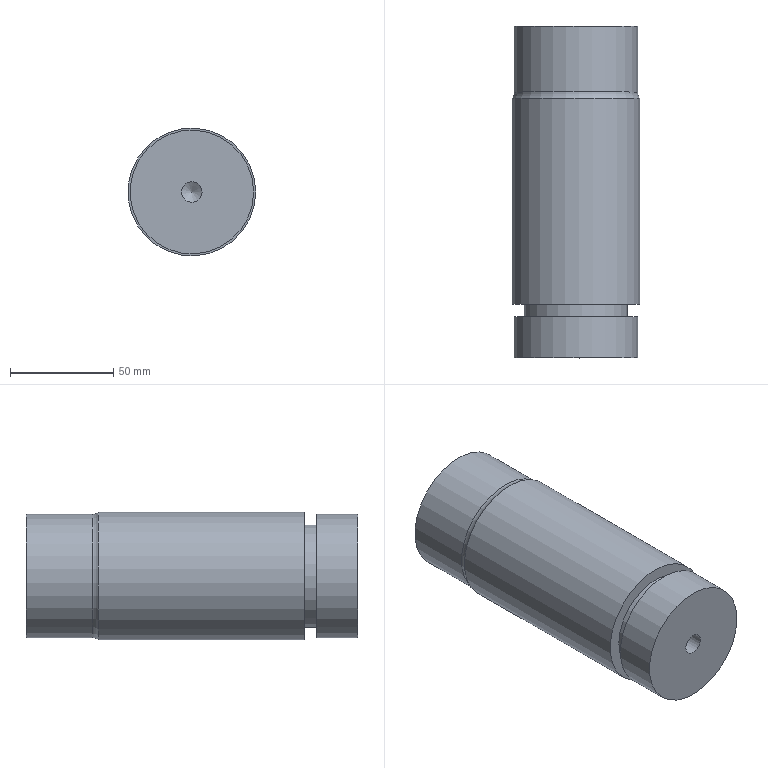Part | NX | features MAIN_BODY 2 | 1 solid | 11 faces | box 62 x 161 x 62 mm | volume 467651 mm3 | cylinder 5 | plane 4 | torus 1 | cone 1 | commonest cylinder face diameters 60 x2 10 x1 50 x1 62 x1
STEP:
#1=CARTESIAN_POINT('',(445.,-617.,262.));
#2=VERTEX_POINT('',#1);
#3=CARTESIAN_POINT('',(414.,-617.,262.));
#4=DIRECTION('',(0.,-1.,0.));
#5=DIRECTION('',(1.,0.,0.));
#6=AXIS2_PLACEMENT_3D('',#3,#4,#5);
#7=CIRCLE('',#6,31.);
#8=EDGE_CURVE('',#2,#2,#7,.T.);
#9=ORIENTED_EDGE('',*,*,#8,.F.);
#10=EDGE_LOOP('',(#9));
#11=FACE_BOUND('',#10,.T.);
#12=CARTESIAN_POINT('',(445.,-517.,262.));
#13=VERTEX_POINT('',#12);
#14=CARTESIAN_POINT('',(414.,-517.,262.));
#15=DIRECTION('',(0.,-1.,0.));
#16=DIRECTION('',(1.,0.,0.));
#17=AXIS2_PLACEMENT_3D('',#14,#15,#16);
#18=CIRCLE('',#17,31.);
#19=EDGE_CURVE('',#13,#13,#18,.T.);
#20=ORIENTED_EDGE('',*,*,#19,.T.);
#21=EDGE_LOOP('',(#20));
#22=FACE_BOUND('',#21,.T.);
#23=CARTESIAN_POINT('',(414.,-617.,262.));
#24=DIRECTION('',(0.,1.,0.));
#25=DIRECTION('',(-1.,0.,0.));
#26=AXIS2_PLACEMENT_3D('',#23,#24,#25);
#27=CYLINDRICAL_SURFACE('',#26,31.);
#28=ADVANCED_FACE('',(#11,#22),#27,.T.);
#29=CARTESIAN_POINT('',(439.,-617.,262.));
#30=VERTEX_POINT('',#29);
#31=CARTESIAN_POINT('',(414.,-617.,262.));
#32=DIRECTION('',(0.,-1.,0.));
#33=DIRECTION('',(1.,0.,0.));
#34=AXIS2_PLACEMENT_3D('',#31,#32,#33);
#35=CIRCLE('',#34,25.);
#36=EDGE_CURVE('',#30,#30,#35,.T.);
#37=ORIENTED_EDGE('',*,*,#36,.F.);
#38=EDGE_LOOP('',(#37));
#39=FACE_BOUND('',#38,.T.);
#40=ORIENTED_EDGE('',*,*,#8,.T.);
#41=EDGE_LOOP('',(#40));
#42=FACE_BOUND('',#41,.T.);
#43=CARTESIAN_POINT('',(414.,-617.,262.));
#44=DIRECTION('',(0.,-1.,0.));
#45=DIRECTION('',(1.,0.,0.));
#46=AXIS2_PLACEMENT_3D('',#43,#44,#45);
#47=PLANE('',#46);
#48=ADVANCED_FACE('',(#39,#42),#47,.T.);
#49=CARTESIAN_POINT('',(444.,-514.,262.));
#50=VERTEX_POINT('',#49);
#51=CARTESIAN_POINT('',(414.,-514.,262.));
#52=DIRECTION('',(0.,-1.,0.));
#53=DIRECTION('',(1.,0.,0.));
#54=AXIS2_PLACEMENT_3D('',#51,#52,#53);
#55=CIRCLE('',#54,30.);
#56=EDGE_CURVE('',#50,#50,#55,.F.);
#57=ORIENTED_EDGE('',*,*,#56,.T.);
#58=EDGE_LOOP('',(#57));
#59=FACE_BOUND('',#58,.T.);
#60=CARTESIAN_POINT('',(444.,-482.,262.));
#61=VERTEX_POINT('',#60);
#62=CARTESIAN_POINT('',(414.,-482.,262.));
#63=DIRECTION('',(0.,-1.,0.));
#64=DIRECTION('',(1.,0.,0.));
#65=AXIS2_PLACEMENT_3D('',#62,#63,#64);
#66=CIRCLE('',#65,30.);
#67=EDGE_CURVE('',#61,#61,#66,.T.);
#68=ORIENTED_EDGE('',*,*,#67,.T.);
#69=EDGE_LOOP('',(#68));
#70=FACE_BOUND('',#69,.T.);
#71=CARTESIAN_POINT('',(414.,-617.,262.));
#72=DIRECTION('',(0.,1.,0.));
#73=DIRECTION('',(-1.,0.,0.));
#74=AXIS2_PLACEMENT_3D('',#71,#72,#73);
#75=CYLINDRICAL_SURFACE('',#74,30.);
#76=ADVANCED_FACE('',(#59,#70),#75,.T.);
#77=ORIENTED_EDGE('',*,*,#67,.F.);
#78=EDGE_LOOP('',(#77));
#79=FACE_BOUND('',#78,.T.);
#80=CARTESIAN_POINT('',(414.,-482.,262.));
#81=DIRECTION('',(0.,-1.,0.));
#82=DIRECTION('',(1.,0.,0.));
#83=AXIS2_PLACEMENT_3D('',#80,#81,#82);
#84=PLANE('',#83);
#85=ADVANCED_FACE('',(#79),#84,.F.);
#86=ORIENTED_EDGE('',*,*,#19,.F.);
#87=EDGE_LOOP('',(#86));
#88=FACE_BOUND('',#87,.T.);
#89=ORIENTED_EDGE('',*,*,#56,.F.);
#90=EDGE_LOOP('',(#89));
#91=FACE_BOUND('',#90,.T.);
#92=CARTESIAN_POINT('',(414.,-514.,262.));
#93=DIRECTION('',(0.,-1.,0.));
#94=DIRECTION('',(1.,0.,0.));
#95=AXIS2_PLACEMENT_3D('',#92,#93,#94);
#96=TOROIDAL_SURFACE('',#95,35.,5.);
#97=ADVANCED_FACE('',(#88,#91),#96,.F.);
#98=ORIENTED_EDGE('',*,*,#36,.T.);
#99=EDGE_LOOP('',(#98));
#100=FACE_BOUND('',#99,.T.);
#101=CARTESIAN_POINT('',(439.,-623.,262.));
#102=VERTEX_POINT('',#101);
#103=CARTESIAN_POINT('',(414.,-623.,262.));
#104=DIRECTION('',(0.,-1.,0.));
#105=DIRECTION('',(1.,0.,0.));
#106=AXIS2_PLACEMENT_3D('',#103,#104,#105);
#107=CIRCLE('',#106,25.);
#108=EDGE_CURVE('',#102,#102,#107,.T.);
#109=ORIENTED_EDGE('',*,*,#108,.F.);
#110=EDGE_LOOP('',(#109));
#111=FACE_BOUND('',#110,.T.);
#112=CARTESIAN_POINT('',(414.,-617.,262.));
#113=DIRECTION('',(0.,-1.,0.));
#114=DIRECTION('',(1.,0.,0.));
#115=AXIS2_PLACEMENT_3D('',#112,#113,#114);
#116=CYLINDRICAL_SURFACE('',#115,25.);
#117=ADVANCED_FACE('',(#100,#111),#116,.T.);
#118=CARTESIAN_POINT('',(444.,-643.,262.));
#119=VERTEX_POINT('',#118);
#120=CARTESIAN_POINT('',(414.,-643.,262.));
#121=DIRECTION('',(0.,-1.,0.));
#122=DIRECTION('',(1.,0.,0.));
#123=AXIS2_PLACEMENT_3D('',#120,#121,#122);
#124=CIRCLE('',#123,30.);
#125=EDGE_CURVE('',#119,#119,#124,.T.);
#126=ORIENTED_EDGE('',*,*,#125,.F.);
#127=EDGE_LOOP('',(#126));
#128=FACE_BOUND('',#127,.T.);
#129=CARTESIAN_POINT('',(444.,-623.,262.));
#130=VERTEX_POINT('',#129);
#131=CARTESIAN_POINT('',(414.,-623.,262.));
#132=DIRECTION('',(0.,-1.,0.));
#133=DIRECTION('',(1.,0.,0.));
#134=AXIS2_PLACEMENT_3D('',#131,#132,#133);
#135=CIRCLE('',#134,30.);
#136=EDGE_CURVE('',#130,#130,#135,.T.);
#137=ORIENTED_EDGE('',*,*,#136,.T.);
#138=EDGE_LOOP('',(#137));
#139=FACE_BOUND('',#138,.T.);
#140=CARTESIAN_POINT('',(414.,-637.,262.));
#141=DIRECTION('',(0.,1.,0.));
#142=DIRECTION('',(-1.,0.,0.));
#143=AXIS2_PLACEMENT_3D('',#140,#141,#142);
#144=CYLINDRICAL_SURFACE('',#143,30.);
#145=ADVANCED_FACE('',(#128,#139),#144,.T.);
#146=CARTESIAN_POINT('',(419.,-643.,262.));
#147=VERTEX_POINT('',#146);
#148=CARTESIAN_POINT('',(414.,-643.,262.));
#149=DIRECTION('',(0.,-1.,0.));
#150=DIRECTION('',(1.,0.,0.));
#151=AXIS2_PLACEMENT_3D('',#148,#149,#150);
#152=CIRCLE('',#151,5.);
#153=EDGE_CURVE('',#147,#147,#152,.F.);
#154=ORIENTED_EDGE('',*,*,#153,.T.);
#155=EDGE_LOOP('',(#154));
#156=FACE_BOUND('',#155,.T.);
#157=ORIENTED_EDGE('',*,*,#125,.T.);
#158=EDGE_LOOP('',(#157));
#159=FACE_BOUND('',#158,.T.);
#160=CARTESIAN_POINT('',(414.,-643.,262.));
#161=DIRECTION('',(0.,-1.,0.));
#162=DIRECTION('',(1.,0.,0.));
#163=AXIS2_PLACEMENT_3D('',#160,#161,#162);
#164=PLANE('',#163);
#165=ADVANCED_FACE('',(#156,#159),#164,.T.);
#166=ORIENTED_EDGE('',*,*,#108,.T.);
#167=EDGE_LOOP('',(#166));
#168=FACE_BOUND('',#167,.T.);
#169=ORIENTED_EDGE('',*,*,#136,.F.);
#170=EDGE_LOOP('',(#169));
#171=FACE_BOUND('',#170,.T.);
#172=CARTESIAN_POINT('',(414.,-623.,262.));
#173=DIRECTION('',(0.,-1.,0.));
#174=DIRECTION('',(1.,0.,0.));
#175=AXIS2_PLACEMENT_3D('',#172,#173,#174);
#176=PLANE('',#175);
#177=ADVANCED_FACE('',(#168,#171),#176,.F.);
#178=CARTESIAN_POINT('',(409.,-622.,262.));
#179=VERTEX_POINT('',#178);
#180=CARTESIAN_POINT('',(414.,-622.,262.));
#181=DIRECTION('',(0.,1.,0.));
#182=DIRECTION('',(-1.,0.,0.));
#183=AXIS2_PLACEMENT_3D('',#180,#181,#182);
#184=CIRCLE('',#183,5.);
#185=EDGE_CURVE('',#179,#179,#184,.T.);
#186=ORIENTED_EDGE('',*,*,#185,.F.);
#187=EDGE_LOOP('',(#186));
#188=FACE_BOUND('',#187,.T.);
#189=CARTESIAN_POINT('',(414.,-618.996,262.));
#190=VERTEX_POINT('',#189);
#191=VERTEX_LOOP('',#190);
#192=FACE_BOUND('',#191,.T.);
#193=CARTESIAN_POINT('',(414.,-622.,262.));
#194=DIRECTION('',(0.,-1.,0.));
#195=DIRECTION('',(1.,0.,0.));
#196=AXIS2_PLACEMENT_3D('',#193,#194,#195);
#197=CONICAL_SURFACE('',#196,5.,1.03);
#198=ADVANCED_FACE('',(#188,#192),#197,.F.);
#199=ORIENTED_EDGE('',*,*,#185,.T.);
#200=EDGE_LOOP('',(#199));
#201=FACE_BOUND('',#200,.T.);
#202=ORIENTED_EDGE('',*,*,#153,.F.);
#203=EDGE_LOOP('',(#202));
#204=FACE_BOUND('',#203,.T.);
#205=CARTESIAN_POINT('',(414.,-637.,262.));
#206=DIRECTION('',(0.,1.,0.));
#207=DIRECTION('',(-1.,0.,0.));
#208=AXIS2_PLACEMENT_3D('',#205,#206,#207);
#209=CYLINDRICAL_SURFACE('',#208,5.);
#210=ADVANCED_FACE('',(#201,#204),#209,.F.);
#211=CLOSED_SHELL('',(#28,#48,#76,#85,#97,#117,#145,#165,#177,#198,#210));
#212=MANIFOLD_SOLID_BREP('',#211);
#213=(LENGTH_UNIT()NAMED_UNIT(*)SI_UNIT(.MILLI.,.METRE.));
#214=UNCERTAINTY_MEASURE_WITH_UNIT(LENGTH_MEASURE(0.00001),#213,'','');
#215=(NAMED_UNIT(*)PLANE_ANGLE_UNIT()SI_UNIT($,.RADIAN.));
#216=(NAMED_UNIT(*)SI_UNIT($,.STERADIAN.)SOLID_ANGLE_UNIT());
#217=(GEOMETRIC_REPRESENTATION_CONTEXT(3)GLOBAL_UNCERTAINTY_ASSIGNED_CONTEXT((#214))GLOBAL_UNIT_ASSIGNED_CONTEXT((#213,#215,#216))REPRESENTATION_CONTEXT('',''));
#218=ADVANCED_BREP_SHAPE_REPRESENTATION('',(#212),#217);